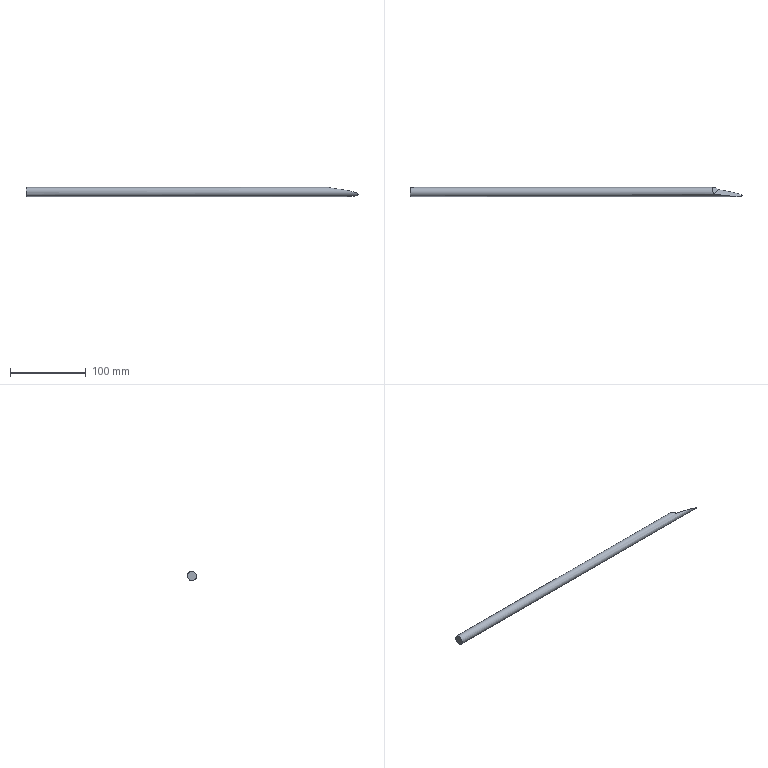Part | STEP file | solid 187 | 1 solid | 5 faces | box 439.33 x 12.005 x 12.001 mm | volume 46615 mm3 | spline 3 | cylinder 1 | plane 1 | commonest cylinder face diameters 12 x1